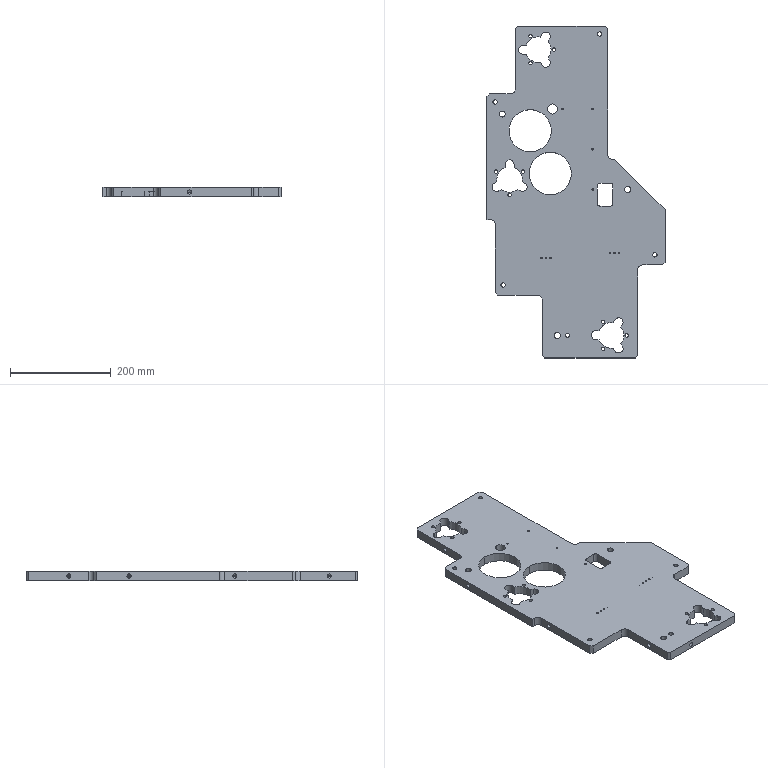NC program | NX | posted with a generic post | part box 354 x 660 x 18 mm
Lines 42876 to 43361 of 43361:
(ZLEVEL_PROFILE_COPY_1 , TOOL : D8JING)
N85738 T09 M6
N85740 G17 G43 G0 G90 X-313.881 Y81.572 Z30. S6000 H9 M3
N85742 Z-17.
N85744 G94 G1 Z-18. F1000.
N85746 Y80.973
N85748 G3 X-313.481 Y80.28 R0.8
N85750 G1 X-308.162 Y77.209
N85752 G2 X-306.215 Y73.097 R4.
N85754 G3 X-292.588 Y49.494 R21.5
N85756 G2 X-290. Y45.751 R4.
N85758 G1 Y39.61
N85760 G3 X-285. Y34.61 R5.
N85762 X-280. Y39.61 R5.
N85764 G1 Y45.751
N85766 G2 X-277.412 Y49.494 R4.
N85768 G3 X-263.785 Y73.097 R21.5
N85770 G2 X-261.838 Y77.209 R4.
N85772 G1 X-256.519 Y80.28
N85774 G3 X-254.689 Y87.11 R5.
N85776 X-261.519 Y88.94 R5.
N85778 G1 X-266.383 Y86.132
N85780 X-266.397 Y86.126
N85782 X-266.655 Y85.981
N85784 G2 X-271.373 Y86.24 R4.
N85786 G3 X-297.936 Y86.783 R21.5
N85788 G1 X-297.994 Y86.729
N85790 X-298.48 Y86.353
N85792 X-298.488 Y86.341
N85794 X-298.497 Y86.351
N85796 G2 X-303.162 Y85.87 R4.
N85798 G1 X-308.481 Y88.94
N85800 G3 X-315.311 Y87.11 R5.
N85802 X-313.481 Y80.28 R5.
N85804 X-312.681 Y80.28 R0.8
N85806 G1 X-312.281 Y80.511
N85808 Z-17.
N85810 G0 Z30.
N85812 X35.82 Y-88.388
N85814 Z-17.
N85816 G1 Z-18.
N85818 X36.057 Y-88.8
N85820 G3 X36.75 Y-89.2 R0.8
N85822 X74.75 Y-51.2 R38.
N85824 X36.75 Y-89.2 R-38.
N85826 X37.443 Y-88.8 R0.8
N85828 G1 X37.68 Y-88.388
N85830 Z-17.
N85832 G0 Z30.
N85834 X13.038 Y-160.881
N85836 Z-17.
N85838 G1 Z-18.
N85840 X13.637
N85842 G3 X14.33 Y-160.481 R0.8
N85844 G1 X17.401 Y-155.162
N85846 G2 X21.513 Y-153.215 R4.
N85848 G3 X45.116 Y-139.588 R21.5
N85850 G2 X49.169 Y-137.012 R4.
N85852 G1 X49.182 Y-137.003
N85854 X49.382 Y-137.
N85856 X55.
N85858 G3 X60. Y-132. R5.
N85860 X55. Y-127. R5.
N85862 G1 X49.394
N85864 X49.194 Y-126.996
N85866 X49.181 Y-126.987
N85868 G2 X45.116 Y-124.412 R4.
N85870 G3 X21.513 Y-110.785 R21.5
N85872 G2 X17.401 Y-108.838 R4.
N85874 G1 X14.33 Y-103.519
N85876 G3 X7.5 Y-101.689 R5.
N85878 X5.67 Y-108.519 R5.
N85880 G1 X8.74 Y-113.838
N85882 G2 X8.254 Y-118.509 R4.
N85884 G1 X8.25 Y-118.528
N85886 X7.926 Y-118.947
N85888 X7.915 Y-118.949
N85890 G3 X8.37 Y-145.627 R21.5
N85892 G2 X8.74 Y-150.162 R4.
N85894 G1 X5.67 Y-155.481
N85896 G3 X7.5 Y-162.311 R5.
N85898 X14.33 Y-160.481 R5.
N85900 X14.33 Y-159.681 R0.8
N85902 G1 X14.099 Y-159.281
N85904 Z-17.
N85906 G0 Z30.
N85908 X120.82 Y-128.388
N85910 Z-17.
N85912 G1 Z-18.
N85914 X121.057 Y-128.8
N85916 G3 X121.75 Y-129.2 R0.8
N85918 X159.75 Y-91.2 R38.
N85920 X121.75 Y-129.2 R-38.
N85922 X122.443 Y-128.8 R0.8
N85924 G1 X122.68 Y-128.388
N85926 Z-17.
N85928 G0 Z30.
N85930 X305.043 Y-67.216
N85932 Z-17.
N85934 G1 Z-18.
N85936 X305.362 Y-67.401
N85938 G3 X306.162 Y-67.401 R0.8
N85940 G1 X311.481 Y-64.33
N85942 G3 X313.311 Y-57.5 R5.
N85944 X306.481 Y-55.67 R5.
N85946 G1 X301.162 Y-58.74
N85948 G2 X296.627 Y-58.37 R4.
N85950 G3 X270.064 Y-57.827 R21.5
N85952 G1 X270.006 Y-57.881
N85954 X269.52 Y-58.257
N85956 X269.512 Y-58.269
N85958 X269.503 Y-58.259
N85960 G2 X264.838 Y-58.74 R4.
N85962 G1 X259.519 Y-55.67
N85964 G3 X252.689 Y-57.5 R5.
N85966 X254.519 Y-64.33 R5.
N85968 G1 X259.838 Y-67.401
N85970 G2 X261.785 Y-71.513 R4.
N85972 G3 X275.412 Y-95.116 R21.5
N85974 G2 X278. Y-98.859 R4.
N85976 G1 Y-105.
N85978 G3 X283. Y-110. R5.
N85980 X288. Y-105. R5.
N85982 G1 Y-98.859
N85984 G2 X290.588 Y-95.116 R4.
N85986 G3 X304.215 Y-71.513 R21.5
N85988 G2 X306.162 Y-67.401 R4.
N85990 G3 X306.562 Y-66.708 R0.8
N85992 G1 Y-66.246
N85994 Z-17.
N85996 G0 Z30.
(FACE_MILLING , TOOL : D8JING)
N85998 M6
N86000 G17 G43 G0 G90 X330. Y69.314 Z30. S6500 H9 M3
N86002 Z3.
N86004 G94 G1 Z0. F1250.
N86006 Y63.657
N86008 Y-121.657
N86010 X326.657 Y-125.
N86012 X326.
N86014 Y67.
N86016 X322.
N86018 Y-125.
N86020 X318.
N86022 Y67.
N86024 X314.
N86026 Y-125.
N86028 X310.
N86030 Y67.
N86032 X306.
N86034 Y-125.
N86036 X302.
N86038 Y67.
N86040 X298.
N86042 Y-125.
N86044 X294.
N86046 Y67.
N86048 X290.
N86050 Y-125.
N86052 X286.
N86054 Y67.
N86056 X282.
N86058 Y-125.
N86060 X278.
N86062 Y67.
N86064 X274.
N86066 Y-125.
N86068 X270.
N86070 Y67.
N86072 X266.
N86074 Y-125.
N86076 X262.
N86078 Y67.
N86080 X258.
N86082 Y-125.
N86084 X254.
N86086 Y67.
N86088 X250.
N86090 Y-125.
N86092 X246.
N86094 Y67.
N86096 X242.
N86098 Y-125.
N86100 X238.
N86102 Y67.
N86104 X234.
N86106 Y-125.
N86108 X230.
N86110 Y67.
N86112 X226.
N86114 Y-125.
N86116 X222.
N86118 Y67.
N86120 X218.
N86122 Y-125.
N86124 X214.
N86126 Y67.
N86128 X210.
N86130 Y-125.
N86132 X206.
N86134 Y67.
N86136 X202.
N86138 Y-125.804
N86140 X199. Y-173.657
N86142 X198. Y-174.657
N86144 Y67.
N86146 X194.
N86148 Y-178.657
N86150 X191.657 Y-181.
N86152 X190.
N86154 Y67.
N86156 X186.
N86158 Y-181.
N86160 X182.
N86162 Y67.
N86164 X178.
N86166 Y-181.
N86168 X174.
N86170 Y67.
N86172 X170.
N86174 Y-181.
N86176 X166.
N86178 Y67.
N86180 X162.
N86182 Y-181.
N86184 X158.
N86186 Y67.
N86188 X154.
N86190 Y-181.
N86192 X150.
N86194 Y67.
N86196 X146.
N86198 Y-181.
N86200 X142.
N86202 Y67.
N86204 X138.
N86206 Y-181.
N86208 X134.
N86210 Y67.
N86212 X130.
N86214 Y-181.
N86216 X126.
N86218 Y67.
N86220 X122.
N86222 Y-181.
N86224 X118.
N86226 Y67.
N86228 X114.
N86230 Y-181.
N86232 X110.
N86234 Y67.
N86236 X106.
N86238 Y-181.
N86240 X102.
N86242 Y67.
N86244 X98.
N86246 Y-181.
N86248 X94.
N86250 Y67.
N86252 X90.
N86254 Y-181.
N86256 X86.
N86258 Y67.
N86260 X82.
N86262 Y-181.
N86264 X78.
N86266 Y67.
N86268 X74. Y67.084
N86270 Y-181.
N86272 X70.
N86274 Y69.683
N86276 X69. Y78.657
N86278 X66. Y81.657
N86280 Y-181.
N86282 X62.
N86284 Y85.657
N86286 X58. Y89.657
N86288 Y-181.
N86290 X54.
N86292 Y93.657
N86294 X50. Y97.657
N86296 Y-181.
N86298 X46.
N86300 Y101.657
N86302 X42. Y105.657
N86304 Y-181.
N86306 X38.
N86308 Y109.657
N86310 X34. Y113.657
N86312 Y-181.
N86314 X30.
N86316 Y117.657
N86318 X26. Y121.657
N86320 Y-181.
N86322 X22.
N86324 Y125.657
N86326 X18. Y129.657
N86328 Y-181.
N86330 X14.
N86332 Y133.657
N86334 X10. Y137.657
N86336 Y-181.
N86338 X6.
N86340 Y141.657
N86342 X2. Y145.657
N86344 Y-181.
N86346 X-2.
N86348 Y149.657
N86350 X-6. Y153.657
N86352 Y-181.
N86354 X-10.
N86356 Y157.657
N86358 X-14. Y161.657
N86360 Y-181.
N86362 X-18.
N86364 Y165.657
N86366 X-22. Y169.657
N86368 Y-181.
N86370 X-26.
N86372 Y173.657
N86374 X-30. Y177.657
N86376 Y-181.
N86378 X-34.
N86380 Y181.
N86382 X-38.
N86384 Y-181.
N86386 X-42.
N86388 Y181.
N86390 X-46.
N86392 Y-181.
N86394 X-50.
N86396 Y181.
N86398 X-54.
N86400 Y-181.
N86402 X-58.
N86404 Y181.
N86406 X-62.
N86408 Y-165.304
N86410 X-66. Y-164.5
N86412 Y181.
N86414 X-70.
N86416 Y-164.5
N86418 X-74.
N86420 Y181.
N86422 X-78.
N86424 Y-164.5
N86426 X-82.
N86428 Y181.
N86430 X-86.
N86432 Y-164.5
N86434 X-90.
N86436 Y181.
N86438 X-94.
N86440 Y-164.5
N86442 X-98.
N86444 Y181.
N86446 X-102.
N86448 Y-164.5
N86450 X-106.
N86452 Y181.
N86454 X-110.
N86456 Y-164.5
N86458 X-114.
N86460 Y181.
N86462 X-118.
N86464 Y-164.5
N86466 X-122.
N86468 Y181.
N86470 X-126.
N86472 Y-164.5
N86474 X-130.
N86476 Y181.
N86478 X-134.
N86480 Y-164.5
N86482 X-138.
N86484 Y181.
N86486 X-141.657
N86488 X-142. Y180.657
N86490 Y-164.5
N86492 X-146.
N86494 Y176.657
N86496 X-149. Y173.657
N86498 X-150. Y129.683
N86500 Y-164.5
N86502 X-154.
N86504 Y127.084
N86506 X-158. Y127.
N86508 Y-164.5
N86510 X-162.
N86512 Y127.
N86514 X-166.
N86516 Y-164.5
N86518 X-170.
N86520 Y127.
N86522 X-174.
N86524 Y-164.5
N86526 X-178.
N86528 Y127.
N86530 X-182.
N86532 Y-164.5
N86534 X-186.
N86536 Y127.
N86538 X-190.
N86540 Y-164.5
N86542 X-194.
N86544 Y127.
N86546 X-198.
N86548 Y-164.5
N86550 X-201.657
N86552 X-202. Y-164.157
N86554 Y127.
N86556 X-206.
N86558 Y-160.157
N86560 X-209. Y-157.157
N86562 X-210. Y-73.683
N86564 Y127.
N86566 X-214.
N86568 Y-71.084
N86570 X-218. Y-71.
N86572 Y127.
N86574 X-222.
N86576 Y-71.
N86578 X-226.
N86580 Y127.
N86582 X-230.
N86584 Y-71.
N86586 X-234.
N86588 Y127.
N86590 X-238.
N86592 Y-71.
N86594 X-242.
N86596 Y127.
N86598 X-246.
N86600 Y-71.
N86602 X-250.
N86604 Y127.
N86606 X-254.
N86608 Y-71.
N86610 X-258.
N86612 Y127.
N86614 X-262.
N86616 Y-71.
N86618 X-266.
N86620 Y127.
N86622 X-270.
N86624 Y-71.
N86626 X-274.
N86628 Y127.
N86630 X-278.
N86632 Y-71.
N86634 X-282.
N86636 Y127.
N86638 X-286.
N86640 Y-71.
N86642 X-290.
N86644 Y127.
N86646 X-294.
N86648 Y-71.
N86650 X-298.
N86652 Y127.
N86654 X-302.
N86656 Y-71.
N86658 X-306.
N86660 Y127.
N86662 X-310.
N86664 Y-71.
N86666 X-314.
N86668 Y127.
N86670 X-318.
N86672 Y-71.
N86674 X-322.
N86676 Y127.
N86678 X-326.
N86680 Y-71.
N86682 X-326.657
N86684 X-330. Y-67.657
N86686 Y123.657
N86688 Y129.314
N86690 Z3.
N86692 G0 Z30.
N86694 M5
N86696 M2